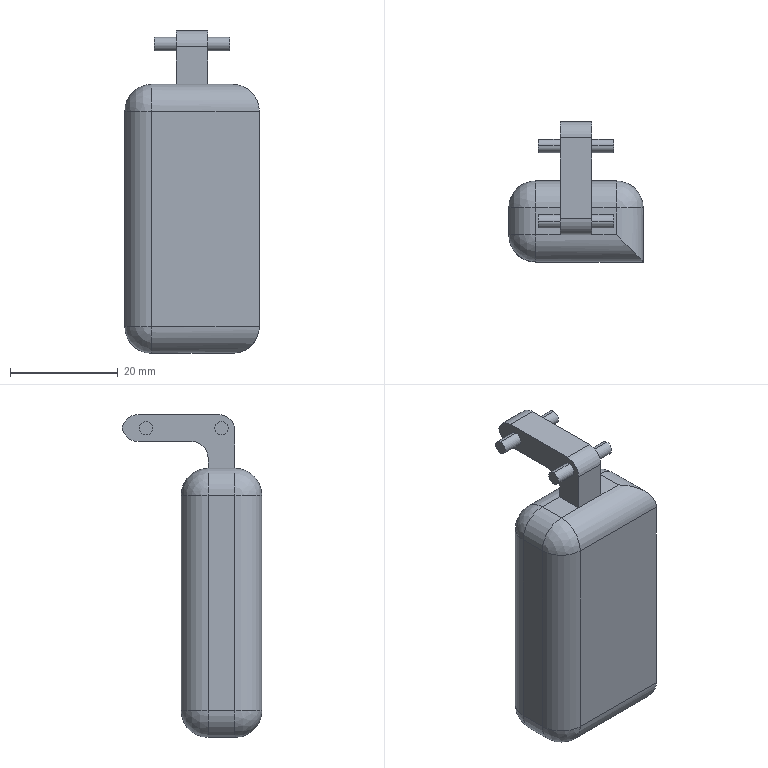Part | SolidWorks | features ICE 3, Fillet 2, Extrusion 1 | 1 solid | 46 faces | box 25 x 25.958 x 60 mm | volume 18052 mm3 | cylinder 23 | plane 17 | sphere 6 | commonest cylinder face diameters 10 x11 2.5 x8 6 x4
STEP:
#1=CARTESIAN_POINT('',(7.,14.,6.255));
#2=VERTEX_POINT('',#1);
#3=CARTESIAN_POINT('',(7.,14.,8.755));
#4=VERTEX_POINT('',#3);
#5=CARTESIAN_POINT('',(7.,14.,7.505));
#6=DIRECTION('',(1.,0.,0.));
#7=DIRECTION('',(0.,0.,-1.));
#8=AXIS2_PLACEMENT_3D('',#5,#6,#7);
#9=CIRCLE('',#8,1.25);
#10=EDGE_CURVE('',#2,#4,#9,.T.);
#11=ORIENTED_EDGE('',*,*,#10,.F.);
#12=CARTESIAN_POINT('',(2.916,14.,6.255));
#13=VERTEX_POINT('',#12);
#14=CARTESIAN_POINT('',(7.,14.,6.255));
#15=DIRECTION('',(-1.,0.,0.));
#16=VECTOR('',#15,1000.);
#17=LINE('',#14,#16);
#18=EDGE_CURVE('',#2,#13,#17,.T.);
#19=ORIENTED_EDGE('',*,*,#18,.T.);
#20=CARTESIAN_POINT('',(2.916,14.,8.755));
#21=VERTEX_POINT('',#20);
#22=CARTESIAN_POINT('',(2.916,14.,7.505));
#23=DIRECTION('',(1.,0.,0.));
#24=DIRECTION('',(0.,0.,1.));
#25=AXIS2_PLACEMENT_3D('',#22,#23,#24);
#26=CIRCLE('',#25,1.25);
#27=EDGE_CURVE('',#13,#21,#26,.T.);
#28=ORIENTED_EDGE('',*,*,#27,.T.);
#29=CARTESIAN_POINT('',(7.,14.,8.755));
#30=DIRECTION('',(-1.,0.,0.));
#31=VECTOR('',#30,1000.);
#32=LINE('',#29,#31);
#33=EDGE_CURVE('',#4,#21,#32,.T.);
#34=ORIENTED_EDGE('',*,*,#33,.F.);
#35=EDGE_LOOP('',(#11,#19,#28,#34));
#36=FACE_OUTER_BOUND('',#35,.T.);
#37=CARTESIAN_POINT('',(7.,14.,7.505));
#38=DIRECTION('',(-1.,0.,0.));
#39=DIRECTION('',(0.,0.,1.));
#40=AXIS2_PLACEMENT_3D('',#37,#38,#39);
#41=CYLINDRICAL_SURFACE('',#40,1.25);
#42=ADVANCED_FACE('',(#36),#41,.T.);
#43=CARTESIAN_POINT('',(-2.916,14.,8.755));
#44=VERTEX_POINT('',#43);
#45=CARTESIAN_POINT('',(-2.916,14.,6.255));
#46=VERTEX_POINT('',#45);
#47=CARTESIAN_POINT('',(-2.916,14.,7.505));
#48=DIRECTION('',(-1.,0.,0.));
#49=DIRECTION('',(0.,0.,-1.));
#50=AXIS2_PLACEMENT_3D('',#47,#48,#49);
#51=CIRCLE('',#50,1.25);
#52=EDGE_CURVE('',#44,#46,#51,.T.);
#53=ORIENTED_EDGE('',*,*,#52,.T.);
#54=CARTESIAN_POINT('',(-7.,14.,6.255));
#55=VERTEX_POINT('',#54);
#56=CARTESIAN_POINT('',(7.,14.,6.255));
#57=DIRECTION('',(-1.,0.,0.));
#58=VECTOR('',#57,1000.);
#59=LINE('',#56,#58);
#60=EDGE_CURVE('',#46,#55,#59,.T.);
#61=ORIENTED_EDGE('',*,*,#60,.T.);
#62=CARTESIAN_POINT('',(-7.,14.,8.755));
#63=VERTEX_POINT('',#62);
#64=CARTESIAN_POINT('',(-7.,14.,7.505));
#65=DIRECTION('',(1.,0.,0.));
#66=DIRECTION('',(0.,0.,-1.));
#67=AXIS2_PLACEMENT_3D('',#64,#65,#66);
#68=CIRCLE('',#67,1.25);
#69=EDGE_CURVE('',#55,#63,#68,.T.);
#70=ORIENTED_EDGE('',*,*,#69,.T.);
#71=CARTESIAN_POINT('',(7.,14.,8.755));
#72=DIRECTION('',(-1.,0.,0.));
#73=VECTOR('',#72,1000.);
#74=LINE('',#71,#73);
#75=EDGE_CURVE('',#44,#63,#74,.T.);
#76=ORIENTED_EDGE('',*,*,#75,.F.);
#77=EDGE_LOOP('',(#53,#61,#70,#76));
#78=FACE_OUTER_BOUND('',#77,.T.);
#79=CARTESIAN_POINT('',(7.,14.,7.505));
#80=DIRECTION('',(-1.,0.,0.));
#81=DIRECTION('',(0.,0.,1.));
#82=AXIS2_PLACEMENT_3D('',#79,#80,#81);
#83=CYLINDRICAL_SURFACE('',#82,1.25);
#84=ADVANCED_FACE('',(#78),#83,.T.);
#85=CARTESIAN_POINT('',(7.,0.,6.255));
#86=VERTEX_POINT('',#85);
#87=CARTESIAN_POINT('',(7.,0.,8.755));
#88=VERTEX_POINT('',#87);
#89=CARTESIAN_POINT('',(7.,0.,7.505));
#90=DIRECTION('',(1.,0.,0.));
#91=DIRECTION('',(0.,0.,-1.));
#92=AXIS2_PLACEMENT_3D('',#89,#90,#91);
#93=CIRCLE('',#92,1.25);
#94=EDGE_CURVE('',#86,#88,#93,.T.);
#95=ORIENTED_EDGE('',*,*,#94,.F.);
#96=CARTESIAN_POINT('',(2.916,0.,6.255));
#97=VERTEX_POINT('',#96);
#98=CARTESIAN_POINT('',(7.,0.,6.255));
#99=DIRECTION('',(-1.,0.,0.));
#100=VECTOR('',#99,1000.);
#101=LINE('',#98,#100);
#102=EDGE_CURVE('',#86,#97,#101,.T.);
#103=ORIENTED_EDGE('',*,*,#102,.T.);
#104=CARTESIAN_POINT('',(2.916,0.,8.755));
#105=VERTEX_POINT('',#104);
#106=CARTESIAN_POINT('',(2.916,0.,7.505));
#107=DIRECTION('',(1.,0.,0.));
#108=DIRECTION('',(0.,0.,1.));
#109=AXIS2_PLACEMENT_3D('',#106,#107,#108);
#110=CIRCLE('',#109,1.25);
#111=EDGE_CURVE('',#97,#105,#110,.T.);
#112=ORIENTED_EDGE('',*,*,#111,.T.);
#113=CARTESIAN_POINT('',(7.,0.,8.755));
#114=DIRECTION('',(-1.,0.,0.));
#115=VECTOR('',#114,1000.);
#116=LINE('',#113,#115);
#117=EDGE_CURVE('',#88,#105,#116,.T.);
#118=ORIENTED_EDGE('',*,*,#117,.F.);
#119=EDGE_LOOP('',(#95,#103,#112,#118));
#120=FACE_OUTER_BOUND('',#119,.T.);
#121=CARTESIAN_POINT('',(7.,0.,7.505));
#122=DIRECTION('',(-1.,0.,0.));
#123=DIRECTION('',(0.,0.,1.));
#124=AXIS2_PLACEMENT_3D('',#121,#122,#123);
#125=CYLINDRICAL_SURFACE('',#124,1.25);
#126=ADVANCED_FACE('',(#120),#125,.T.);
#127=CARTESIAN_POINT('',(-2.916,0.,8.755));
#128=VERTEX_POINT('',#127);
#129=CARTESIAN_POINT('',(-2.916,0.,6.255));
#130=VERTEX_POINT('',#129);
#131=CARTESIAN_POINT('',(-2.916,0.,7.505));
#132=DIRECTION('',(-1.,0.,0.));
#133=DIRECTION('',(0.,0.,-1.));
#134=AXIS2_PLACEMENT_3D('',#131,#132,#133);
#135=CIRCLE('',#134,1.25);
#136=EDGE_CURVE('',#128,#130,#135,.T.);
#137=ORIENTED_EDGE('',*,*,#136,.T.);
#138=CARTESIAN_POINT('',(-7.,0.,6.255));
#139=VERTEX_POINT('',#138);
#140=CARTESIAN_POINT('',(7.,0.,6.255));
#141=DIRECTION('',(-1.,0.,0.));
#142=VECTOR('',#141,1000.);
#143=LINE('',#140,#142);
#144=EDGE_CURVE('',#130,#139,#143,.T.);
#145=ORIENTED_EDGE('',*,*,#144,.T.);
#146=CARTESIAN_POINT('',(-7.,0.,8.755));
#147=VERTEX_POINT('',#146);
#148=CARTESIAN_POINT('',(-7.,0.,7.505));
#149=DIRECTION('',(1.,0.,0.));
#150=DIRECTION('',(0.,0.,-1.));
#151=AXIS2_PLACEMENT_3D('',#148,#149,#150);
#152=CIRCLE('',#151,1.25);
#153=EDGE_CURVE('',#139,#147,#152,.T.);
#154=ORIENTED_EDGE('',*,*,#153,.T.);
#155=CARTESIAN_POINT('',(7.,0.,8.755));
#156=DIRECTION('',(-1.,0.,0.));
#157=VECTOR('',#156,1000.);
#158=LINE('',#155,#157);
#159=EDGE_CURVE('',#128,#147,#158,.T.);
#160=ORIENTED_EDGE('',*,*,#159,.F.);
#161=EDGE_LOOP('',(#137,#145,#154,#160));
#162=FACE_OUTER_BOUND('',#161,.T.);
#163=CARTESIAN_POINT('',(7.,0.,7.505));
#164=DIRECTION('',(-1.,0.,0.));
#165=DIRECTION('',(0.,0.,1.));
#166=AXIS2_PLACEMENT_3D('',#163,#164,#165);
#167=CYLINDRICAL_SURFACE('',#166,1.25);
#168=ADVANCED_FACE('',(#162),#167,.T.);
#169=CARTESIAN_POINT('',(-2.916,2.5,2.));
#170=VERTEX_POINT('',#169);
#171=CARTESIAN_POINT('',(-2.916,2.5,0.));
#172=VERTEX_POINT('',#171);
#173=CARTESIAN_POINT('',(-2.916,2.5,10.));
#174=DIRECTION('',(0.,0.,-1.));
#175=VECTOR('',#174,1000.);
#176=LINE('',#173,#175);
#177=EDGE_CURVE('',#170,#172,#176,.T.);
#178=ORIENTED_EDGE('',*,*,#177,.F.);
#179=CARTESIAN_POINT('',(2.916,2.5,2.));
#180=VERTEX_POINT('',#179);
#181=CARTESIAN_POINT('',(2.916,2.5,2.));
#182=DIRECTION('',(1.,0.,0.));
#183=VECTOR('',#182,1000.);
#184=LINE('',#181,#183);
#185=EDGE_CURVE('',#170,#180,#184,.T.);
#186=ORIENTED_EDGE('',*,*,#185,.T.);
#187=CARTESIAN_POINT('',(2.916,2.5,0.));
#188=VERTEX_POINT('',#187);
#189=CARTESIAN_POINT('',(2.916,2.5,10.));
#190=DIRECTION('',(0.,0.,-1.));
#191=VECTOR('',#190,1000.);
#192=LINE('',#189,#191);
#193=EDGE_CURVE('',#180,#188,#192,.T.);
#194=ORIENTED_EDGE('',*,*,#193,.T.);
#195=CARTESIAN_POINT('',(-2.916,2.5,0.));
#196=DIRECTION('',(-1.,0.,0.));
#197=VECTOR('',#196,1000.);
#198=LINE('',#195,#197);
#199=EDGE_CURVE('',#188,#172,#198,.T.);
#200=ORIENTED_EDGE('',*,*,#199,.T.);
#201=EDGE_LOOP('',(#178,#186,#194,#200));
#202=FACE_OUTER_BOUND('',#201,.T.);
#203=CARTESIAN_POINT('',(-2.916,2.5,10.));
#204=DIRECTION('',(0.,-1.,0.));
#205=DIRECTION('',(0.,0.,-1.));
#206=AXIS2_PLACEMENT_3D('',#203,#204,#205);
#207=PLANE('',#206);
#208=ADVANCED_FACE('',(#202),#207,.F.);
#209=CARTESIAN_POINT('',(7.5,2.5,0.));
#210=VERTEX_POINT('',#209);
#211=CARTESIAN_POINT('',(0.,2.5,0.));
#212=DIRECTION('',(-1.,0.,0.));
#213=VECTOR('',#212,1000.);
#214=LINE('',#211,#213);
#215=EDGE_CURVE('',#210,#188,#214,.T.);
#216=ORIENTED_EDGE('',*,*,#215,.T.);
#217=CARTESIAN_POINT('',(2.916,-2.5,0.));
#218=VERTEX_POINT('',#217);
#219=CARTESIAN_POINT('',(2.916,2.5,0.));
#220=DIRECTION('',(0.,1.,0.));
#221=VECTOR('',#220,1000.);
#222=LINE('',#219,#221);
#223=EDGE_CURVE('',#218,#188,#222,.T.);
#224=ORIENTED_EDGE('',*,*,#223,.F.);
#225=CARTESIAN_POINT('',(7.5,-2.5,0.));
#226=VERTEX_POINT('',#225);
#227=CARTESIAN_POINT('',(0.,-2.5,0.));
#228=DIRECTION('',(1.,0.,0.));
#229=VECTOR('',#228,1000.);
#230=LINE('',#227,#229);
#231=EDGE_CURVE('',#218,#226,#230,.T.);
#232=ORIENTED_EDGE('',*,*,#231,.T.);
#233=CARTESIAN_POINT('',(7.5,0.,0.));
#234=DIRECTION('',(0.,1.,0.));
#235=VECTOR('',#234,1000.);
#236=LINE('',#233,#235);
#237=EDGE_CURVE('',#226,#210,#236,.T.);
#238=ORIENTED_EDGE('',*,*,#237,.T.);
#239=EDGE_LOOP('',(#216,#224,#232,#238));
#240=FACE_OUTER_BOUND('',#239,.T.);
#241=CARTESIAN_POINT('',(0.,0.,0.));
#242=DIRECTION('',(0.,0.,1.));
#243=DIRECTION('',(1.,0.,0.));
#244=AXIS2_PLACEMENT_3D('',#241,#242,#243);
#245=PLANE('',#244);
#246=ADVANCED_FACE('',(#240),#245,.T.);
#247=CARTESIAN_POINT('',(-7.5,-2.5,0.));
#248=VERTEX_POINT('',#247);
#249=CARTESIAN_POINT('',(-2.916,-2.5,0.));
#250=VERTEX_POINT('',#249);
#251=CARTESIAN_POINT('',(0.,-2.5,0.));
#252=DIRECTION('',(1.,0.,0.));
#253=VECTOR('',#252,1000.);
#254=LINE('',#251,#253);
#255=EDGE_CURVE('',#248,#250,#254,.T.);
#256=ORIENTED_EDGE('',*,*,#255,.T.);
#257=CARTESIAN_POINT('',(-2.916,2.5,0.));
#258=DIRECTION('',(0.,-1.,0.));
#259=VECTOR('',#258,1000.);
#260=LINE('',#257,#259);
#261=EDGE_CURVE('',#172,#250,#260,.T.);
#262=ORIENTED_EDGE('',*,*,#261,.F.);
#263=CARTESIAN_POINT('',(-7.5,2.5,0.));
#264=VERTEX_POINT('',#263);
#265=CARTESIAN_POINT('',(0.,2.5,0.));
#266=DIRECTION('',(-1.,0.,0.));
#267=VECTOR('',#266,1000.);
#268=LINE('',#265,#267);
#269=EDGE_CURVE('',#172,#264,#268,.T.);
#270=ORIENTED_EDGE('',*,*,#269,.T.);
#271=CARTESIAN_POINT('',(-7.5,0.,0.));
#272=DIRECTION('',(0.,-1.,0.));
#273=VECTOR('',#272,1000.);
#274=LINE('',#271,#273);
#275=EDGE_CURVE('',#264,#248,#274,.T.);
#276=ORIENTED_EDGE('',*,*,#275,.T.);
#277=EDGE_LOOP('',(#256,#262,#270,#276));
#278=FACE_OUTER_BOUND('',#277,.T.);
#279=CARTESIAN_POINT('',(0.,0.,0.));
#280=DIRECTION('',(0.,0.,1.));
#281=DIRECTION('',(1.,0.,0.));
#282=AXIS2_PLACEMENT_3D('',#279,#280,#281);
#283=PLANE('',#282);
#284=ADVANCED_FACE('',(#278),#283,.T.);
#285=CARTESIAN_POINT('',(12.5,2.5,-45.));
#286=VERTEX_POINT('',#285);
#287=CARTESIAN_POINT('',(12.5,2.5,-5.));
#288=VERTEX_POINT('',#287);
#289=CARTESIAN_POINT('',(12.5,2.5,-50.));
#290=DIRECTION('',(0.,0.,1.));
#291=VECTOR('',#290,1000.);
#292=LINE('',#289,#291);
#293=EDGE_CURVE('',#286,#288,#292,.T.);
#294=ORIENTED_EDGE('',*,*,#293,.T.);
#295=CARTESIAN_POINT('',(12.5,-7.5,-5.));
#296=VERTEX_POINT('',#295);
#297=CARTESIAN_POINT('',(12.5,7.5,-5.));
#298=DIRECTION('',(0.,-1.,0.));
#299=VECTOR('',#298,1000.);
#300=LINE('',#297,#299);
#301=EDGE_CURVE('',#288,#296,#300,.T.);
#302=ORIENTED_EDGE('',*,*,#301,.T.);
#303=CARTESIAN_POINT('',(12.5,-7.5,-45.));
#304=VERTEX_POINT('',#303);
#305=CARTESIAN_POINT('',(12.5,-7.5,-50.));
#306=DIRECTION('',(0.,0.,1.));
#307=VECTOR('',#306,1000.);
#308=LINE('',#305,#307);
#309=EDGE_CURVE('',#304,#296,#308,.T.);
#310=ORIENTED_EDGE('',*,*,#309,.F.);
#311=CARTESIAN_POINT('',(12.5,7.5,-45.));
#312=DIRECTION('',(0.,1.,0.));
#313=VECTOR('',#312,1000.);
#314=LINE('',#311,#313);
#315=EDGE_CURVE('',#304,#286,#314,.T.);
#316=ORIENTED_EDGE('',*,*,#315,.T.);
#317=EDGE_LOOP('',(#294,#302,#310,#316));
#318=FACE_OUTER_BOUND('',#317,.T.);
#319=CARTESIAN_POINT('',(12.5,7.5,-50.));
#320=DIRECTION('',(1.,0.,0.));
#321=DIRECTION('',(0.,1.,0.));
#322=AXIS2_PLACEMENT_3D('',#319,#320,#321);
#323=PLANE('',#322);
#324=ADVANCED_FACE('',(#318),#323,.T.);
#325=ORIENTED_EDGE('',*,*,#309,.T.);
#326=CARTESIAN_POINT('',(-7.5,-7.5,-5.));
#327=VERTEX_POINT('',#326);
#328=CARTESIAN_POINT('',(-12.5,-7.5,-5.));
#329=DIRECTION('',(-1.,0.,0.));
#330=VECTOR('',#329,1000.);
#331=LINE('',#328,#330);
#332=EDGE_CURVE('',#296,#327,#331,.T.);
#333=ORIENTED_EDGE('',*,*,#332,.T.);
#334=CARTESIAN_POINT('',(-7.5,-7.5,-45.));
#335=VERTEX_POINT('',#334);
#336=CARTESIAN_POINT('',(-7.5,-7.5,-50.));
#337=DIRECTION('',(0.,0.,-1.));
#338=VECTOR('',#337,1000.);
#339=LINE('',#336,#338);
#340=EDGE_CURVE('',#327,#335,#339,.T.);
#341=ORIENTED_EDGE('',*,*,#340,.T.);
#342=CARTESIAN_POINT('',(12.5,-7.5,-45.));
#343=DIRECTION('',(1.,0.,0.));
#344=VECTOR('',#343,1000.);
#345=LINE('',#342,#344);
#346=EDGE_CURVE('',#335,#304,#345,.T.);
#347=ORIENTED_EDGE('',*,*,#346,.T.);
#348=EDGE_LOOP('',(#325,#333,#341,#347));
#349=FACE_OUTER_BOUND('',#348,.T.);
#350=CARTESIAN_POINT('',(-12.5,-7.5,-50.));
#351=DIRECTION('',(0.,-1.,0.));
#352=DIRECTION('',(0.,0.,-1.));
#353=AXIS2_PLACEMENT_3D('',#350,#351,#352);
#354=PLANE('',#353);
#355=ADVANCED_FACE('',(#349),#354,.T.);
#356=CARTESIAN_POINT('',(-12.5,-2.5,-45.));
#357=VERTEX_POINT('',#356);
#358=CARTESIAN_POINT('',(-12.5,-2.5,-5.));
#359=VERTEX_POINT('',#358);
#360=CARTESIAN_POINT('',(-12.5,-2.5,-50.));
#361=DIRECTION('',(0.,0.,1.));
#362=VECTOR('',#361,1000.);
#363=LINE('',#360,#362);
#364=EDGE_CURVE('',#357,#359,#363,.T.);
#365=ORIENTED_EDGE('',*,*,#364,.T.);
#366=CARTESIAN_POINT('',(-12.5,2.5,-5.));
#367=VERTEX_POINT('',#366);
#368=CARTESIAN_POINT('',(-12.5,7.5,-5.));
#369=DIRECTION('',(0.,1.,0.));
#370=VECTOR('',#369,1000.);
#371=LINE('',#368,#370);
#372=EDGE_CURVE('',#359,#367,#371,.T.);
#373=ORIENTED_EDGE('',*,*,#372,.T.);
#374=CARTESIAN_POINT('',(-12.5,2.5,-45.));
#375=VERTEX_POINT('',#374);
#376=CARTESIAN_POINT('',(-12.5,2.5,-50.));
#377=DIRECTION('',(0.,0.,-1.));
#378=VECTOR('',#377,1000.);
#379=LINE('',#376,#378);
#380=EDGE_CURVE('',#367,#375,#379,.T.);
#381=ORIENTED_EDGE('',*,*,#380,.T.);
#382=CARTESIAN_POINT('',(-12.5,-7.5,-45.));
#383=DIRECTION('',(0.,-1.,0.));
#384=VECTOR('',#383,1000.);
#385=LINE('',#382,#384);
#386=EDGE_CURVE('',#375,#357,#385,.T.);
#387=ORIENTED_EDGE('',*,*,#386,.T.);
#388=EDGE_LOOP('',(#365,#373,#381,#387));
#389=FACE_OUTER_BOUND('',#388,.T.);
#390=CARTESIAN_POINT('',(-12.5,7.5,-50.));
#391=DIRECTION('',(-1.,0.,0.));
#392=DIRECTION('',(0.,-1.,0.));
#393=AXIS2_PLACEMENT_3D('',#390,#391,#392);
#394=PLANE('',#393);
#395=ADVANCED_FACE('',(#389),#394,.T.);
#396=CARTESIAN_POINT('',(7.5,7.5,-45.));
#397=VERTEX_POINT('',#396);
#398=CARTESIAN_POINT('',(-7.5,7.5,-45.));
#399=VERTEX_POINT('',#398);
#400=CARTESIAN_POINT('',(-12.5,7.5,-45.));
#401=DIRECTION('',(-1.,0.,0.));
#402=VECTOR('',#401,1000.);
#403=LINE('',#400,#402);
#404=EDGE_CURVE('',#397,#399,#403,.T.);
#405=ORIENTED_EDGE('',*,*,#404,.T.);
#406=CARTESIAN_POINT('',(-7.5,7.5,-5.));
#407=VERTEX_POINT('',#406);
#408=CARTESIAN_POINT('',(-7.5,7.5,-50.));
#409=DIRECTION('',(0.,0.,1.));
#410=VECTOR('',#409,1000.);
#411=LINE('',#408,#410);
#412=EDGE_CURVE('',#399,#407,#411,.T.);
#413=ORIENTED_EDGE('',*,*,#412,.T.);
#414=CARTESIAN_POINT('',(7.5,7.5,-5.));
#415=VERTEX_POINT('',#414);
#416=CARTESIAN_POINT('',(-12.5,7.5,-5.));
#417=DIRECTION('',(1.,0.,0.));
#418=VECTOR('',#417,1000.);
#419=LINE('',#416,#418);
#420=EDGE_CURVE('',#407,#415,#419,.T.);
#421=ORIENTED_EDGE('',*,*,#420,.T.);
#422=CARTESIAN_POINT('',(7.5,7.5,-50.));
#423=DIRECTION('',(0.,0.,-1.));
#424=VECTOR('',#423,1000.);
#425=LINE('',#422,#424);
#426=EDGE_CURVE('',#415,#397,#425,.T.);
#427=ORIENTED_EDGE('',*,*,#426,.T.);
#428=EDGE_LOOP('',(#405,#413,#421,#427));
#429=FACE_OUTER_BOUND('',#428,.T.);
#430=CARTESIAN_POINT('',(-12.5,7.5,-50.));
#431=DIRECTION('',(0.,1.,0.));
#432=DIRECTION('',(0.,0.,1.));
#433=AXIS2_PLACEMENT_3D('',#430,#431,#432);
#434=PLANE('',#433);
#435=ADVANCED_FACE('',(#429),#434,.T.);
#436=CARTESIAN_POINT('',(7.5,2.5,-50.));
#437=VERTEX_POINT('',#436);
#438=CARTESIAN_POINT('',(7.5,-2.5,-50.));
#439=VERTEX_POINT('',#438);
#440=CARTESIAN_POINT('',(7.5,-7.5,-50.));
#441=DIRECTION('',(0.,-1.,0.));
#442=VECTOR('',#441,1000.);
#443=LINE('',#440,#442);
#444=EDGE_CURVE('',#437,#439,#443,.T.);
#445=ORIENTED_EDGE('',*,*,#444,.T.);
#446=CARTESIAN_POINT('',(-7.5,-2.5,-50.));
#447=VERTEX_POINT('',#446);
#448=CARTESIAN_POINT('',(-12.5,-2.5,-50.));
#449=DIRECTION('',(-1.,0.,0.));
#450=VECTOR('',#449,1000.);
#451=LINE('',#448,#450);
#452=EDGE_CURVE('',#439,#447,#451,.T.);
#453=ORIENTED_EDGE('',*,*,#452,.T.);
#454=CARTESIAN_POINT('',(-7.5,2.5,-50.));
#455=VERTEX_POINT('',#454);
#456=CARTESIAN_POINT('',(-7.5,7.5,-50.));
#457=DIRECTION('',(0.,1.,0.));
#458=VECTOR('',#457,1000.);
#459=LINE('',#456,#458);
#460=EDGE_CURVE('',#447,#455,#459,.T.);
#461=ORIENTED_EDGE('',*,*,#460,.T.);
#462=CARTESIAN_POINT('',(12.5,2.5,-50.));
#463=DIRECTION('',(1.,0.,0.));
#464=VECTOR('',#463,1000.);
#465=LINE('',#462,#464);
#466=EDGE_CURVE('',#455,#437,#465,.T.);
#467=ORIENTED_EDGE('',*,*,#466,.T.);
#468=EDGE_LOOP('',(#445,#453,#461,#467));
#469=FACE_OUTER_BOUND('',#468,.T.);
#470=CARTESIAN_POINT('',(0.,0.,-50.));
#471=DIRECTION('',(0.,0.,1.));
#472=DIRECTION('',(1.,0.,0.));
#473=AXIS2_PLACEMENT_3D('',#470,#471,#472);
#474=PLANE('',#473);
#475=ADVANCED_FACE('',(#469),#474,.F.);
#476=CARTESIAN_POINT('',(7.5,2.5,-45.));
#477=DIRECTION('',(0.,0.,1.));
#478=DIRECTION('',(-1.,0.,0.));
#479=AXIS2_PLACEMENT_3D('',#476,#477,#478);
#480=CIRCLE('',#479,5.);
#481=EDGE_CURVE('',#286,#397,#480,.T.);
#482=ORIENTED_EDGE('',*,*,#481,.F.);
#483=CARTESIAN_POINT('',(7.5,2.5,-45.));
#484=DIRECTION('',(0.,-1.,0.));
#485=DIRECTION('',(-1.,0.,0.));
#486=AXIS2_PLACEMENT_3D('',#483,#484,#485);
#487=CIRCLE('',#486,5.);
#488=EDGE_CURVE('',#437,#286,#487,.T.);
#489=ORIENTED_EDGE('',*,*,#488,.F.);
#490=CARTESIAN_POINT('',(7.5,2.5,-45.));
#491=DIRECTION('',(-1.,0.,0.));
#492=DIRECTION('',(0.,0.,-1.));
#493=AXIS2_PLACEMENT_3D('',#490,#491,#492);
#494=CIRCLE('',#493,5.);
#495=EDGE_CURVE('',#397,#437,#494,.T.);
#496=ORIENTED_EDGE('',*,*,#495,.F.);
#497=EDGE_LOOP('',(#482,#489,#496));
#498=FACE_OUTER_BOUND('',#497,.T.);
#499=CARTESIAN_POINT('',(7.5,2.5,-45.));
#500=DIRECTION('',(0.,1.,0.));
#501=DIRECTION('',(-1.,0.,0.));
#502=AXIS2_PLACEMENT_3D('',#499,#500,#501);
#503=SPHERICAL_SURFACE('',#502,5.);
#504=ADVANCED_FACE('',(#498),#503,.T.);
#505=ORIENTED_EDGE('',*,*,#488,.T.);
#506=ORIENTED_EDGE('',*,*,#315,.F.);
#507=CARTESIAN_POINT('',(7.5,-2.5,-50.));
#508=CARTESIAN_POINT('',(10.429,-5.429,-50.));
#509=CARTESIAN_POINT('',(12.5,-7.5,-47.929));
#510=CARTESIAN_POINT('',(12.5,-7.5,-45.));
#511=(BOUNDED_CURVE()B_SPLINE_CURVE(3,(#507,#508,#509,#510),.UNSPECIFIED.,.F.,.T.)B_SPLINE_CURVE_WITH_KNOTS((4,4),(4.712,6.283),.UNSPECIFIED.)CURVE()GEOMETRIC_REPRESENTATION_ITEM()RATIONAL_B_SPLINE_CURVE((1.,0.8047,0.8047,1.))REPRESENTATION_ITEM(''));
#512=EDGE_CURVE('',#439,#304,#511,.T.);
#513=ORIENTED_EDGE('',*,*,#512,.F.);
#514=ORIENTED_EDGE('',*,*,#444,.F.);
#515=EDGE_LOOP('',(#505,#506,#513,#514));
#516=FACE_OUTER_BOUND('',#515,.T.);
#517=CARTESIAN_POINT('',(7.5,7.5,-45.));
#518=DIRECTION('',(0.,-1.,0.));
#519=DIRECTION('',(1.,0.,0.));
#520=AXIS2_PLACEMENT_3D('',#517,#518,#519);
#521=CYLINDRICAL_SURFACE('',#520,5.);
#522=ADVANCED_FACE('',(#516),#521,.T.);
#523=ORIENTED_EDGE('',*,*,#495,.T.);
#524=ORIENTED_EDGE('',*,*,#466,.F.);
#525=CARTESIAN_POINT('',(-7.5,2.5,-45.));
#526=DIRECTION('',(-1.,0.,0.));
#527=DIRECTION('',(0.,0.,1.));
#528=AXIS2_PLACEMENT_3D('',#525,#526,#527);
#529=CIRCLE('',#528,5.);
#530=EDGE_CURVE('',#399,#455,#529,.T.);
#531=ORIENTED_EDGE('',*,*,#530,.F.);
#532=ORIENTED_EDGE('',*,*,#404,.F.);
#533=EDGE_LOOP('',(#523,#524,#531,#532));
#534=FACE_OUTER_BOUND('',#533,.T.);
#535=CARTESIAN_POINT('',(-12.5,2.5,-45.));
#536=DIRECTION('',(1.,0.,0.));
#537=DIRECTION('',(0.,0.,-1.));
#538=AXIS2_PLACEMENT_3D('',#535,#536,#537);
#539=CYLINDRICAL_SURFACE('',#538,5.);
#540=ADVANCED_FACE('',(#534),#539,.T.);
#541=ORIENTED_EDGE('',*,*,#481,.T.);
#542=ORIENTED_EDGE('',*,*,#426,.F.);
#543=CARTESIAN_POINT('',(7.5,2.5,-5.));
#544=DIRECTION('',(0.,0.,1.));
#545=DIRECTION('',(1.,0.,0.));
#546=AXIS2_PLACEMENT_3D('',#543,#544,#545);
#547=CIRCLE('',#546,5.);
#548=EDGE_CURVE('',#288,#415,#547,.T.);
#549=ORIENTED_EDGE('',*,*,#548,.F.);
#550=ORIENTED_EDGE('',*,*,#293,.F.);
#551=EDGE_LOOP('',(#541,#542,#549,#550));
#552=FACE_OUTER_BOUND('',#551,.T.);
#553=CARTESIAN_POINT('',(7.5,2.5,-50.));
#554=DIRECTION('',(0.,0.,1.));
#555=DIRECTION('',(1.,0.,0.));
#556=AXIS2_PLACEMENT_3D('',#553,#554,#555);
#557=CYLINDRICAL_SURFACE('',#556,5.);
#558=ADVANCED_FACE('',(#552),#557,.T.);
#559=ORIENTED_EDGE('',*,*,#512,.T.);
#560=ORIENTED_EDGE('',*,*,#346,.F.);
#561=CARTESIAN_POINT('',(-7.5,-2.5,-45.));
#562=DIRECTION('',(-1.,0.,0.));
#563=DIRECTION('',(0.,0.,1.));
#564=AXIS2_PLACEMENT_3D('',#561,#562,#563);
#565=CIRCLE('',#564,5.);
#566=EDGE_CURVE('',#447,#335,#565,.T.);
#567=ORIENTED_EDGE('',*,*,#566,.F.);
#568=ORIENTED_EDGE('',*,*,#452,.F.);
#569=EDGE_LOOP('',(#559,#560,#567,#568));
#570=FACE_OUTER_BOUND('',#569,.T.);
#571=CARTESIAN_POINT('',(-12.5,-2.5,-45.));
#572=DIRECTION('',(-1.,0.,0.));
#573=DIRECTION('',(0.,0.,1.));
#574=AXIS2_PLACEMENT_3D('',#571,#572,#573);
#575=CYLINDRICAL_SURFACE('',#574,5.);
#576=ADVANCED_FACE('',(#570),#575,.T.);
#577=CARTESIAN_POINT('',(-7.5,2.5,-45.));
#578=DIRECTION('',(0.,1.,0.));
#579=DIRECTION('',(-1.,0.,0.));
#580=AXIS2_PLACEMENT_3D('',#577,#578,#579);
#581=CIRCLE('',#580,5.);
#582=EDGE_CURVE('',#455,#375,#581,.T.);
#583=ORIENTED_EDGE('',*,*,#582,.F.);
#584=ORIENTED_EDGE('',*,*,#460,.F.);
#585=CARTESIAN_POINT('',(-7.5,-2.5,-45.));
#586=DIRECTION('',(0.,-1.,0.));
#587=DIRECTION('',(1.,0.,0.));
#588=AXIS2_PLACEMENT_3D('',#585,#586,#587);
#589=CIRCLE('',#588,5.);
#590=EDGE_CURVE('',#357,#447,#589,.T.);
#591=ORIENTED_EDGE('',*,*,#590,.F.);
#592=ORIENTED_EDGE('',*,*,#386,.F.);
#593=EDGE_LOOP('',(#583,#584,#591,#592));
#594=FACE_OUTER_BOUND('',#593,.T.);
#595=CARTESIAN_POINT('',(-7.5,7.5,-45.));
#596=DIRECTION('',(0.,1.,0.));
#597=DIRECTION('',(-1.,0.,0.));
#598=AXIS2_PLACEMENT_3D('',#595,#596,#597);
#599=CYLINDRICAL_SURFACE('',#598,5.);
#600=ADVANCED_FACE('',(#594),#599,.T.);
#601=ORIENTED_EDGE('',*,*,#530,.T.);
#602=ORIENTED_EDGE('',*,*,#582,.T.);
#603=CARTESIAN_POINT('',(-7.5,2.5,-45.));
#604=DIRECTION('',(0.,0.,1.));
#605=DIRECTION('',(-1.,0.,0.));
#606=AXIS2_PLACEMENT_3D('',#603,#604,#605);
#607=CIRCLE('',#606,5.);
#608=EDGE_CURVE('',#399,#375,#607,.T.);
#609=ORIENTED_EDGE('',*,*,#608,.F.);
#610=EDGE_LOOP('',(#601,#602,#609));
#611=FACE_OUTER_BOUND('',#610,.T.);
#612=CARTESIAN_POINT('',(-7.5,2.5,-45.));
#613=DIRECTION('',(0.,1.,0.));
#614=DIRECTION('',(-1.,0.,0.));
#615=AXIS2_PLACEMENT_3D('',#612,#613,#614);
#616=SPHERICAL_SURFACE('',#615,5.);
#617=ADVANCED_FACE('',(#611),#616,.T.);
#618=CARTESIAN_POINT('',(7.5,2.5,-5.));
#619=DIRECTION('',(-1.,0.,0.));
#620=DIRECTION('',(0.,0.,-1.));
#621=AXIS2_PLACEMENT_3D('',#618,#619,#620);
#622=CIRCLE('',#621,5.);
#623=EDGE_CURVE('',#210,#415,#622,.T.);
#624=ORIENTED_EDGE('',*,*,#623,.F.);
#625=CARTESIAN_POINT('',(7.5,2.5,-5.));
#626=DIRECTION('',(0.,-1.,0.));
#627=DIRECTION('',(-1.,0.,0.));
#628=AXIS2_PLACEMENT_3D('',#625,#626,#627);
#629=CIRCLE('',#628,5.);
#630=EDGE_CURVE('',#288,#210,#629,.T.);
#631=ORIENTED_EDGE('',*,*,#630,.F.);
#632=ORIENTED_EDGE('',*,*,#548,.T.);
#633=EDGE_LOOP('',(#624,#631,#632));
#634=FACE_OUTER_BOUND('',#633,.T.);
#635=CARTESIAN_POINT('',(7.5,2.5,-5.));
#636=DIRECTION('',(0.,0.,1.));
#637=DIRECTION('',(0.,1.,0.));
#638=AXIS2_PLACEMENT_3D('',#635,#636,#637);
#639=SPHERICAL_SURFACE('',#638,5.);
#640=ADVANCED_FACE('',(#634),#639,.T.);
#641=ORIENTED_EDGE('',*,*,#630,.T.);
#642=ORIENTED_EDGE('',*,*,#237,.F.);
#643=CARTESIAN_POINT('',(12.5,-7.5,-5.));
#644=CARTESIAN_POINT('',(12.5,-7.5,-2.071));
#645=CARTESIAN_POINT('',(10.429,-5.429,0.));
#646=CARTESIAN_POINT('',(7.5,-2.5,0.));
#647=(BOUNDED_CURVE()B_SPLINE_CURVE(3,(#643,#644,#645,#646),.UNSPECIFIED.,.F.,.F.)B_SPLINE_CURVE_WITH_KNOTS((4,4),(3.142,4.712),.UNSPECIFIED.)CURVE()GEOMETRIC_REPRESENTATION_ITEM()RATIONAL_B_SPLINE_CURVE((1.,0.8047,0.8047,1.))REPRESENTATION_ITEM(''));
#648=EDGE_CURVE('',#296,#226,#647,.T.);
#649=ORIENTED_EDGE('',*,*,#648,.F.);
#650=ORIENTED_EDGE('',*,*,#301,.F.);
#651=EDGE_LOOP('',(#641,#642,#649,#650));
#652=FACE_OUTER_BOUND('',#651,.T.);
#653=CARTESIAN_POINT('',(7.5,0.,-5.));
#654=DIRECTION('',(0.,1.,0.));
#655=DIRECTION('',(-1.,0.,0.));
#656=AXIS2_PLACEMENT_3D('',#653,#654,#655);
#657=CYLINDRICAL_SURFACE('',#656,5.);
#658=ADVANCED_FACE('',(#652),#657,.T.);
#659=ORIENTED_EDGE('',*,*,#590,.T.);
#660=ORIENTED_EDGE('',*,*,#566,.T.);
#661=CARTESIAN_POINT('',(-7.5,-2.5,-45.));
#662=DIRECTION('',(0.,0.,1.));
#663=DIRECTION('',(-1.,0.,0.));
#664=AXIS2_PLACEMENT_3D('',#661,#662,#663);
#665=CIRCLE('',#664,5.);
#666=EDGE_CURVE('',#357,#335,#665,.T.);
#667=ORIENTED_EDGE('',*,*,#666,.F.);
#668=EDGE_LOOP('',(#659,#660,#667));
#669=FACE_OUTER_BOUND('',#668,.T.);
#670=CARTESIAN_POINT('',(-7.5,-2.5,-45.));
#671=DIRECTION('',(0.,1.,0.));
#672=DIRECTION('',(-1.,0.,0.));
#673=AXIS2_PLACEMENT_3D('',#670,#671,#672);
#674=SPHERICAL_SURFACE('',#673,5.);
#675=ADVANCED_FACE('',(#669),#674,.T.);
#676=ORIENTED_EDGE('',*,*,#608,.T.);
#677=ORIENTED_EDGE('',*,*,#380,.F.);
#678=CARTESIAN_POINT('',(-7.5,2.5,-5.));
#679=DIRECTION('',(0.,0.,1.));
#680=DIRECTION('',(1.,0.,0.));
#681=AXIS2_PLACEMENT_3D('',#678,#679,#680);
#682=CIRCLE('',#681,5.);
#683=EDGE_CURVE('',#407,#367,#682,.T.);
#684=ORIENTED_EDGE('',*,*,#683,.F.);
#685=ORIENTED_EDGE('',*,*,#412,.F.);
#686=EDGE_LOOP('',(#676,#677,#684,#685));
#687=FACE_OUTER_BOUND('',#686,.T.);
#688=CARTESIAN_POINT('',(-7.5,2.5,-50.));
#689=DIRECTION('',(0.,0.,1.));
#690=DIRECTION('',(1.,0.,0.));
#691=AXIS2_PLACEMENT_3D('',#688,#689,#690);
#692=CYLINDRICAL_SURFACE('',#691,5.);
#693=ADVANCED_FACE('',(#687),#692,.T.);
#694=ORIENTED_EDGE('',*,*,#623,.T.);
#695=ORIENTED_EDGE('',*,*,#420,.F.);
#696=CARTESIAN_POINT('',(-7.5,2.5,-5.));
#697=DIRECTION('',(-1.,0.,0.));
#698=DIRECTION('',(0.,0.,1.));
#699=AXIS2_PLACEMENT_3D('',#696,#697,#698);
#700=CIRCLE('',#699,5.);
#701=EDGE_CURVE('',#264,#407,#700,.T.);
#702=ORIENTED_EDGE('',*,*,#701,.F.);
#703=ORIENTED_EDGE('',*,*,#269,.F.);
#704=ORIENTED_EDGE('',*,*,#199,.F.);
#705=ORIENTED_EDGE('',*,*,#215,.F.);
#706=EDGE_LOOP('',(#694,#695,#702,#703,#704,#705));
#707=FACE_OUTER_BOUND('',#706,.T.);
#708=CARTESIAN_POINT('',(0.,2.5,-5.));
#709=DIRECTION('',(-1.,0.,0.));
#710=DIRECTION('',(0.,0.,1.));
#711=AXIS2_PLACEMENT_3D('',#708,#709,#710);
#712=CYLINDRICAL_SURFACE('',#711,5.);
#713=ADVANCED_FACE('',(#707),#712,.T.);
#714=ORIENTED_EDGE('',*,*,#648,.T.);
#715=ORIENTED_EDGE('',*,*,#231,.F.);
#716=CARTESIAN_POINT('',(-2.916,-2.5,0.));
#717=DIRECTION('',(1.,0.,0.));
#718=VECTOR('',#717,1000.);
#719=LINE('',#716,#718);
#720=EDGE_CURVE('',#250,#218,#719,.T.);
#721=ORIENTED_EDGE('',*,*,#720,.F.);
#722=ORIENTED_EDGE('',*,*,#255,.F.);
#723=CARTESIAN_POINT('',(-7.5,-2.5,-5.));
#724=DIRECTION('',(-1.,0.,0.));
#725=DIRECTION('',(0.,0.,1.));
#726=AXIS2_PLACEMENT_3D('',#723,#724,#725);
#727=CIRCLE('',#726,5.);
#728=EDGE_CURVE('',#327,#248,#727,.T.);
#729=ORIENTED_EDGE('',*,*,#728,.F.);
#730=ORIENTED_EDGE('',*,*,#332,.F.);
#731=EDGE_LOOP('',(#714,#715,#721,#722,#729,#730));
#732=FACE_OUTER_BOUND('',#731,.T.);
#733=CARTESIAN_POINT('',(0.,-2.5,-5.));
#734=DIRECTION('',(1.,0.,0.));
#735=DIRECTION('',(0.,0.,-1.));
#736=AXIS2_PLACEMENT_3D('',#733,#734,#735);
#737=CYLINDRICAL_SURFACE('',#736,5.);
#738=ADVANCED_FACE('',(#732),#737,.T.);
#739=ORIENTED_EDGE('',*,*,#666,.T.);
#740=ORIENTED_EDGE('',*,*,#340,.F.);
#741=CARTESIAN_POINT('',(-7.5,-2.5,-5.));
#742=DIRECTION('',(0.,0.,1.));
#743=DIRECTION('',(1.,0.,0.));
#744=AXIS2_PLACEMENT_3D('',#741,#742,#743);
#745=CIRCLE('',#744,5.);
#746=EDGE_CURVE('',#359,#327,#745,.T.);
#747=ORIENTED_EDGE('',*,*,#746,.F.);
#748=ORIENTED_EDGE('',*,*,#364,.F.);
#749=EDGE_LOOP('',(#739,#740,#747,#748));
#750=FACE_OUTER_BOUND('',#749,.T.);
#751=CARTESIAN_POINT('',(-7.5,-2.5,-50.));
#752=DIRECTION('',(0.,0.,1.));
#753=DIRECTION('',(1.,0.,0.));
#754=AXIS2_PLACEMENT_3D('',#751,#752,#753);
#755=CYLINDRICAL_SURFACE('',#754,5.);
#756=ADVANCED_FACE('',(#750),#755,.T.);
#757=ORIENTED_EDGE('',*,*,#701,.T.);
#758=ORIENTED_EDGE('',*,*,#683,.T.);
#759=CARTESIAN_POINT('',(-7.5,2.5,-5.));
#760=DIRECTION('',(0.,-1.,0.));
#761=DIRECTION('',(-1.,0.,0.));
#762=AXIS2_PLACEMENT_3D('',#759,#760,#761);
#763=CIRCLE('',#762,5.);
#764=EDGE_CURVE('',#264,#367,#763,.T.);
#765=ORIENTED_EDGE('',*,*,#764,.F.);
#766=EDGE_LOOP('',(#757,#758,#765));
#767=FACE_OUTER_BOUND('',#766,.T.);
#768=CARTESIAN_POINT('',(-7.5,2.5,-5.));
#769=DIRECTION('',(1.,0.,0.));
#770=DIRECTION('',(0.,0.,1.));
#771=AXIS2_PLACEMENT_3D('',#768,#769,#770);
#772=SPHERICAL_SURFACE('',#771,5.);
#773=ADVANCED_FACE('',(#767),#772,.T.);
#774=ORIENTED_EDGE('',*,*,#746,.T.);
#775=ORIENTED_EDGE('',*,*,#728,.T.);
#776=CARTESIAN_POINT('',(-7.5,-2.5,-5.));
#777=DIRECTION('',(0.,1.,0.));
#778=DIRECTION('',(1.,0.,0.));
#779=AXIS2_PLACEMENT_3D('',#776,#777,#778);
#780=CIRCLE('',#779,5.);
#781=EDGE_CURVE('',#359,#248,#780,.T.);
#782=ORIENTED_EDGE('',*,*,#781,.F.);
#783=EDGE_LOOP('',(#774,#775,#782));
#784=FACE_OUTER_BOUND('',#783,.T.);
#785=CARTESIAN_POINT('',(-7.5,-2.5,-5.));
#786=DIRECTION('',(1.,0.,0.));
#787=DIRECTION('',(0.,0.,-1.));
#788=AXIS2_PLACEMENT_3D('',#785,#786,#787);
#789=SPHERICAL_SURFACE('',#788,5.);
#790=ADVANCED_FACE('',(#784),#789,.T.);
#791=ORIENTED_EDGE('',*,*,#764,.T.);
#792=ORIENTED_EDGE('',*,*,#372,.F.);
#793=ORIENTED_EDGE('',*,*,#781,.T.);
#794=ORIENTED_EDGE('',*,*,#275,.F.);
#795=EDGE_LOOP('',(#791,#792,#793,#794));
#796=FACE_OUTER_BOUND('',#795,.T.);
#797=CARTESIAN_POINT('',(-7.5,0.,-5.));
#798=DIRECTION('',(0.,-1.,0.));
#799=DIRECTION('',(1.,0.,0.));
#800=AXIS2_PLACEMENT_3D('',#797,#798,#799);
#801=CYLINDRICAL_SURFACE('',#800,5.);
#802=ADVANCED_FACE('',(#796),#801,.T.);
#803=CARTESIAN_POINT('',(2.916,14.,7.505));
#804=DIRECTION('',(1.,0.,0.));
#805=DIRECTION('',(0.,0.,1.));
#806=AXIS2_PLACEMENT_3D('',#803,#804,#805);
#807=CIRCLE('',#806,1.25);
#808=EDGE_CURVE('',#21,#13,#807,.T.);
#809=ORIENTED_EDGE('',*,*,#808,.F.);
#810=ORIENTED_EDGE('',*,*,#27,.F.);
#811=EDGE_LOOP('',(#809,#810));
#812=FACE_BOUND('',#811,.T.);
#813=CARTESIAN_POINT('',(2.916,0.,7.505));
#814=DIRECTION('',(1.,0.,0.));
#815=DIRECTION('',(0.,0.,1.));
#816=AXIS2_PLACEMENT_3D('',#813,#814,#815);
#817=CIRCLE('',#816,1.25);
#818=EDGE_CURVE('',#105,#97,#817,.T.);
#819=ORIENTED_EDGE('',*,*,#818,.F.);
#820=ORIENTED_EDGE('',*,*,#111,.F.);
#821=EDGE_LOOP('',(#819,#820));
#822=FACE_BOUND('',#821,.T.);
#823=CARTESIAN_POINT('',(2.916,0.5,10.));
#824=VERTEX_POINT('',#823);
#825=CARTESIAN_POINT('',(2.916,15.5,10.));
#826=VERTEX_POINT('',#825);
#827=CARTESIAN_POINT('',(2.916,2.5,10.));
#828=DIRECTION('',(0.,1.,0.));
#829=VECTOR('',#828,1000.);
#830=LINE('',#827,#829);
#831=EDGE_CURVE('',#824,#826,#830,.T.);
#832=ORIENTED_EDGE('',*,*,#831,.F.);
#833=CARTESIAN_POINT('',(2.916,-2.5,7.));
#834=VERTEX_POINT('',#833);
#835=CARTESIAN_POINT('',(2.916,0.5,7.));
#836=DIRECTION('',(1.,0.,0.));
#837=DIRECTION('',(0.,0.,1.));
#838=AXIS2_PLACEMENT_3D('',#835,#836,#837);
#839=CIRCLE('',#838,3.);
#840=EDGE_CURVE('',#824,#834,#839,.T.);
#841=ORIENTED_EDGE('',*,*,#840,.T.);
#842=CARTESIAN_POINT('',(2.916,-2.5,10.));
#843=DIRECTION('',(0.,0.,-1.));
#844=VECTOR('',#843,1000.);
#845=LINE('',#842,#844);
#846=EDGE_CURVE('',#834,#218,#845,.T.);
#847=ORIENTED_EDGE('',*,*,#846,.T.);
#848=ORIENTED_EDGE('',*,*,#223,.T.);
#849=ORIENTED_EDGE('',*,*,#193,.F.);
#850=CARTESIAN_POINT('',(2.916,5.5,5.));
#851=VERTEX_POINT('',#850);
#852=CARTESIAN_POINT('',(2.916,5.5,2.));
#853=DIRECTION('',(-1.,0.,0.));
#854=DIRECTION('',(0.,0.,1.));
#855=AXIS2_PLACEMENT_3D('',#852,#853,#854);
#856=CIRCLE('',#855,3.);
#857=EDGE_CURVE('',#180,#851,#856,.T.);
#858=ORIENTED_EDGE('',*,*,#857,.T.);
#859=CARTESIAN_POINT('',(2.916,15.5,5.));
#860=VERTEX_POINT('',#859);
#861=CARTESIAN_POINT('',(2.916,18.5,5.));
#862=DIRECTION('',(0.,-1.,0.));
#863=VECTOR('',#862,1000.);
#864=LINE('',#861,#863);
#865=EDGE_CURVE('',#860,#851,#864,.T.);
#866=ORIENTED_EDGE('',*,*,#865,.F.);
#867=CARTESIAN_POINT('',(2.916,18.458,7.5));
#868=VERTEX_POINT('',#867);
#869=CARTESIAN_POINT('',(2.916,15.5,8.));
#870=DIRECTION('',(1.,0.,0.));
#871=DIRECTION('',(0.,0.,1.));
#872=AXIS2_PLACEMENT_3D('',#869,#870,#871);
#873=CIRCLE('',#872,3.);
#874=EDGE_CURVE('',#860,#868,#873,.T.);
#875=ORIENTED_EDGE('',*,*,#874,.T.);
#876=CARTESIAN_POINT('',(2.916,15.5,7.));
#877=DIRECTION('',(1.,0.,0.));
#878=DIRECTION('',(0.,0.,1.));
#879=AXIS2_PLACEMENT_3D('',#876,#877,#878);
#880=CIRCLE('',#879,3.);
#881=EDGE_CURVE('',#868,#826,#880,.T.);
#882=ORIENTED_EDGE('',*,*,#881,.T.);
#883=EDGE_LOOP('',(#832,#841,#847,#848,#849,#858,#866,#875,#882));
#884=FACE_OUTER_BOUND('',#883,.T.);
#885=CARTESIAN_POINT('',(2.916,2.5,10.));
#886=DIRECTION('',(-1.,0.,0.));
#887=DIRECTION('',(0.,0.,1.));
#888=AXIS2_PLACEMENT_3D('',#885,#886,#887);
#889=PLANE('',#888);
#890=ADVANCED_FACE('',(#812,#822,#884),#889,.F.);
#891=ORIENTED_EDGE('',*,*,#52,.F.);
#892=CARTESIAN_POINT('',(-2.916,14.,7.505));
#893=DIRECTION('',(-1.,0.,0.));
#894=DIRECTION('',(0.,0.,-1.));
#895=AXIS2_PLACEMENT_3D('',#892,#893,#894);
#896=CIRCLE('',#895,1.25);
#897=EDGE_CURVE('',#46,#44,#896,.T.);
#898=ORIENTED_EDGE('',*,*,#897,.F.);
#899=EDGE_LOOP('',(#891,#898));
#900=FACE_BOUND('',#899,.T.);
#901=ORIENTED_EDGE('',*,*,#136,.F.);
#902=CARTESIAN_POINT('',(-2.916,0.,7.505));
#903=DIRECTION('',(-1.,0.,0.));
#904=DIRECTION('',(0.,0.,-1.));
#905=AXIS2_PLACEMENT_3D('',#902,#903,#904);
#906=CIRCLE('',#905,1.25);
#907=EDGE_CURVE('',#130,#128,#906,.T.);
#908=ORIENTED_EDGE('',*,*,#907,.F.);
#909=EDGE_LOOP('',(#901,#908));
#910=FACE_BOUND('',#909,.T.);
#911=CARTESIAN_POINT('',(-2.916,-2.5,7.));
#912=VERTEX_POINT('',#911);
#913=CARTESIAN_POINT('',(-2.916,-2.5,10.));
#914=DIRECTION('',(0.,0.,-1.));
#915=VECTOR('',#914,1000.);
#916=LINE('',#913,#915);
#917=EDGE_CURVE('',#912,#250,#916,.T.);
#918=ORIENTED_EDGE('',*,*,#917,.F.);
#919=CARTESIAN_POINT('',(-2.916,0.5,10.));
#920=VERTEX_POINT('',#919);
#921=CARTESIAN_POINT('',(-2.916,0.5,7.));
#922=DIRECTION('',(-1.,0.,0.));
#923=DIRECTION('',(0.,0.,-1.));
#924=AXIS2_PLACEMENT_3D('',#921,#922,#923);
#925=CIRCLE('',#924,3.);
#926=EDGE_CURVE('',#912,#920,#925,.T.);
#927=ORIENTED_EDGE('',*,*,#926,.T.);
#928=CARTESIAN_POINT('',(-2.916,15.5,10.));
#929=VERTEX_POINT('',#928);
#930=CARTESIAN_POINT('',(-2.916,2.5,10.));
#931=DIRECTION('',(0.,-1.,0.));
#932=VECTOR('',#931,1000.);
#933=LINE('',#930,#932);
#934=EDGE_CURVE('',#929,#920,#933,.T.);
#935=ORIENTED_EDGE('',*,*,#934,.F.);
#936=CARTESIAN_POINT('',(-2.916,18.458,7.5));
#937=VERTEX_POINT('',#936);
#938=CARTESIAN_POINT('',(-2.916,15.5,7.));
#939=DIRECTION('',(-1.,0.,0.));
#940=DIRECTION('',(0.,0.,-1.));
#941=AXIS2_PLACEMENT_3D('',#938,#939,#940);
#942=CIRCLE('',#941,3.);
#943=EDGE_CURVE('',#929,#937,#942,.T.);
#944=ORIENTED_EDGE('',*,*,#943,.T.);
#945=CARTESIAN_POINT('',(-2.916,15.5,5.));
#946=VERTEX_POINT('',#945);
#947=CARTESIAN_POINT('',(-2.916,15.5,8.));
#948=DIRECTION('',(-1.,0.,0.));
#949=DIRECTION('',(0.,0.,-1.));
#950=AXIS2_PLACEMENT_3D('',#947,#948,#949);
#951=CIRCLE('',#950,3.);
#952=EDGE_CURVE('',#937,#946,#951,.T.);
#953=ORIENTED_EDGE('',*,*,#952,.T.);
#954=CARTESIAN_POINT('',(-2.916,5.5,5.));
#955=VERTEX_POINT('',#954);
#956=CARTESIAN_POINT('',(-2.916,18.5,5.));
#957=DIRECTION('',(0.,-1.,0.));
#958=VECTOR('',#957,1000.);
#959=LINE('',#956,#958);
#960=EDGE_CURVE('',#946,#955,#959,.T.);
#961=ORIENTED_EDGE('',*,*,#960,.T.);
#962=CARTESIAN_POINT('',(-2.916,5.5,2.));
#963=DIRECTION('',(1.,0.,0.));
#964=DIRECTION('',(0.,0.,-1.));
#965=AXIS2_PLACEMENT_3D('',#962,#963,#964);
#966=CIRCLE('',#965,3.);
#967=EDGE_CURVE('',#955,#170,#966,.T.);
#968=ORIENTED_EDGE('',*,*,#967,.T.);
#969=ORIENTED_EDGE('',*,*,#177,.T.);
#970=ORIENTED_EDGE('',*,*,#261,.T.);
#971=EDGE_LOOP('',(#918,#927,#935,#944,#953,#961,#968,#969,#970));
#972=FACE_OUTER_BOUND('',#971,.T.);
#973=CARTESIAN_POINT('',(-2.916,2.5,10.));
#974=DIRECTION('',(1.,0.,0.));
#975=DIRECTION('',(0.,0.,-1.));
#976=AXIS2_PLACEMENT_3D('',#973,#974,#975);
#977=PLANE('',#976);
#978=ADVANCED_FACE('',(#900,#910,#972),#977,.F.);
#979=ORIENTED_EDGE('',*,*,#846,.F.);
#980=CARTESIAN_POINT('',(-2.916,-2.5,7.));
#981=DIRECTION('',(-1.,0.,0.));
#982=VECTOR('',#981,1000.);
#983=LINE('',#980,#982);
#984=EDGE_CURVE('',#834,#912,#983,.T.);
#985=ORIENTED_EDGE('',*,*,#984,.T.);
#986=ORIENTED_EDGE('',*,*,#917,.T.);
#987=ORIENTED_EDGE('',*,*,#720,.T.);
#988=EDGE_LOOP('',(#979,#985,#986,#987));
#989=FACE_OUTER_BOUND('',#988,.T.);
#990=CARTESIAN_POINT('',(-2.916,-2.5,10.));
#991=DIRECTION('',(0.,1.,0.));
#992=DIRECTION('',(0.,0.,1.));
#993=AXIS2_PLACEMENT_3D('',#990,#991,#992);
#994=PLANE('',#993);
#995=ADVANCED_FACE('',(#989),#994,.F.);
#996=ORIENTED_EDGE('',*,*,#934,.T.);
#997=CARTESIAN_POINT('',(2.916,0.5,10.));
#998=DIRECTION('',(1.,0.,0.));
#999=VECTOR('',#998,1000.);
#1000=LINE('',#997,#999);
#1001=EDGE_CURVE('',#920,#824,#1000,.T.);
#1002=ORIENTED_EDGE('',*,*,#1001,.T.);
#1003=ORIENTED_EDGE('',*,*,#831,.T.);
#1004=CARTESIAN_POINT('',(-2.916,15.5,10.));
#1005=DIRECTION('',(-1.,0.,0.));
#1006=VECTOR('',#1005,1000.);
#1007=LINE('',#1004,#1006);
#1008=EDGE_CURVE('',#826,#929,#1007,.T.);
#1009=ORIENTED_EDGE('',*,*,#1008,.T.);
#1010=EDGE_LOOP('',(#996,#1002,#1003,#1009));
#1011=FACE_OUTER_BOUND('',#1010,.T.);
#1012=CARTESIAN_POINT('',(0.,0.,10.));
#1013=DIRECTION('',(0.,0.,1.));
#1014=DIRECTION('',(1.,0.,0.));
#1015=AXIS2_PLACEMENT_3D('',#1012,#1013,#1014);
#1016=PLANE('',#1015);
#1017=ADVANCED_FACE('',(#1011),#1016,.T.);
#1018=ORIENTED_EDGE('',*,*,#865,.T.);
#1019=CARTESIAN_POINT('',(-2.916,5.5,5.));
#1020=DIRECTION('',(-1.,0.,0.));
#1021=VECTOR('',#1020,1000.);
#1022=LINE('',#1019,#1021);
#1023=EDGE_CURVE('',#851,#955,#1022,.T.);
#1024=ORIENTED_EDGE('',*,*,#1023,.T.);
#1025=ORIENTED_EDGE('',*,*,#960,.F.);
#1026=CARTESIAN_POINT('',(-2.916,15.5,5.));
#1027=DIRECTION('',(1.,0.,0.));
#1028=VECTOR('',#1027,1000.);
#1029=LINE('',#1026,#1028);
#1030=EDGE_CURVE('',#946,#860,#1029,.T.);
#1031=ORIENTED_EDGE('',*,*,#1030,.T.);
#1032=EDGE_LOOP('',(#1018,#1024,#1025,#1031));
#1033=FACE_OUTER_BOUND('',#1032,.T.);
#1034=CARTESIAN_POINT('',(-2.916,18.5,5.));
#1035=DIRECTION('',(0.,0.,1.));
#1036=DIRECTION('',(1.,0.,0.));
#1037=AXIS2_PLACEMENT_3D('',#1034,#1035,#1036);
#1038=PLANE('',#1037);
#1039=ADVANCED_FACE('',(#1033),#1038,.F.);
#1040=CARTESIAN_POINT('',(-7.,0.,7.505));
#1041=DIRECTION('',(1.,0.,0.));
#1042=DIRECTION('',(0.,0.,-1.));
#1043=AXIS2_PLACEMENT_3D('',#1040,#1041,#1042);
#1044=CIRCLE('',#1043,1.25);
#1045=EDGE_CURVE('',#147,#139,#1044,.T.);
#1046=ORIENTED_EDGE('',*,*,#1045,.F.);
#1047=ORIENTED_EDGE('',*,*,#153,.F.);
#1048=EDGE_LOOP('',(#1046,#1047));
#1049=FACE_OUTER_BOUND('',#1048,.T.);
#1050=CARTESIAN_POINT('',(-7.,0.,7.505));
#1051=DIRECTION('',(1.,0.,0.));
#1052=DIRECTION('',(0.,0.,-1.));
#1053=AXIS2_PLACEMENT_3D('',#1050,#1051,#1052);
#1054=PLANE('',#1053);
#1055=ADVANCED_FACE('',(#1049),#1054,.F.);
#1056=ORIENTED_EDGE('',*,*,#144,.F.);
#1057=ORIENTED_EDGE('',*,*,#907,.T.);
#1058=ORIENTED_EDGE('',*,*,#159,.T.);
#1059=ORIENTED_EDGE('',*,*,#1045,.T.);
#1060=EDGE_LOOP('',(#1056,#1057,#1058,#1059));
#1061=FACE_OUTER_BOUND('',#1060,.T.);
#1062=CARTESIAN_POINT('',(7.,0.,7.505));
#1063=DIRECTION('',(-1.,0.,0.));
#1064=DIRECTION('',(0.,0.,1.));
#1065=AXIS2_PLACEMENT_3D('',#1062,#1063,#1064);
#1066=CYLINDRICAL_SURFACE('',#1065,1.25);
#1067=ADVANCED_FACE('',(#1061),#1066,.T.);
#1068=ORIENTED_EDGE('',*,*,#102,.F.);
#1069=CARTESIAN_POINT('',(7.,0.,7.505));
#1070=DIRECTION('',(1.,0.,0.));
#1071=DIRECTION('',(0.,0.,-1.));
#1072=AXIS2_PLACEMENT_3D('',#1069,#1070,#1071);
#1073=CIRCLE('',#1072,1.25);
#1074=EDGE_CURVE('',#88,#86,#1073,.T.);
#1075=ORIENTED_EDGE('',*,*,#1074,.F.);
#1076=ORIENTED_EDGE('',*,*,#117,.T.);
#1077=ORIENTED_EDGE('',*,*,#818,.T.);
#1078=EDGE_LOOP('',(#1068,#1075,#1076,#1077));
#1079=FACE_OUTER_BOUND('',#1078,.T.);
#1080=CARTESIAN_POINT('',(7.,0.,7.505));
#1081=DIRECTION('',(-1.,0.,0.));
#1082=DIRECTION('',(0.,0.,1.));
#1083=AXIS2_PLACEMENT_3D('',#1080,#1081,#1082);
#1084=CYLINDRICAL_SURFACE('',#1083,1.25);
#1085=ADVANCED_FACE('',(#1079),#1084,.T.);
#1086=ORIENTED_EDGE('',*,*,#1074,.T.);
#1087=ORIENTED_EDGE('',*,*,#94,.T.);
#1088=EDGE_LOOP('',(#1086,#1087));
#1089=FACE_OUTER_BOUND('',#1088,.T.);
#1090=CARTESIAN_POINT('',(7.,0.,7.505));
#1091=DIRECTION('',(1.,0.,0.));
#1092=DIRECTION('',(0.,0.,-1.));
#1093=AXIS2_PLACEMENT_3D('',#1090,#1091,#1092);
#1094=PLANE('',#1093);
#1095=ADVANCED_FACE('',(#1089),#1094,.T.);
#1096=CARTESIAN_POINT('',(-7.,14.,7.505));
#1097=DIRECTION('',(1.,0.,0.));
#1098=DIRECTION('',(0.,0.,-1.));
#1099=AXIS2_PLACEMENT_3D('',#1096,#1097,#1098);
#1100=CIRCLE('',#1099,1.25);
#1101=EDGE_CURVE('',#63,#55,#1100,.T.);
#1102=ORIENTED_EDGE('',*,*,#1101,.F.);
#1103=ORIENTED_EDGE('',*,*,#69,.F.);
#1104=EDGE_LOOP('',(#1102,#1103));
#1105=FACE_OUTER_BOUND('',#1104,.T.);
#1106=CARTESIAN_POINT('',(-7.,14.,7.505));
#1107=DIRECTION('',(1.,0.,0.));
#1108=DIRECTION('',(0.,0.,-1.));
#1109=AXIS2_PLACEMENT_3D('',#1106,#1107,#1108);
#1110=PLANE('',#1109);
#1111=ADVANCED_FACE('',(#1105),#1110,.F.);
#1112=ORIENTED_EDGE('',*,*,#60,.F.);
#1113=ORIENTED_EDGE('',*,*,#897,.T.);
#1114=ORIENTED_EDGE('',*,*,#75,.T.);
#1115=ORIENTED_EDGE('',*,*,#1101,.T.);
#1116=EDGE_LOOP('',(#1112,#1113,#1114,#1115));
#1117=FACE_OUTER_BOUND('',#1116,.T.);
#1118=CARTESIAN_POINT('',(7.,14.,7.505));
#1119=DIRECTION('',(-1.,0.,0.));
#1120=DIRECTION('',(0.,0.,1.));
#1121=AXIS2_PLACEMENT_3D('',#1118,#1119,#1120);
#1122=CYLINDRICAL_SURFACE('',#1121,1.25);
#1123=ADVANCED_FACE('',(#1117),#1122,.T.);
#1124=ORIENTED_EDGE('',*,*,#18,.F.);
#1125=CARTESIAN_POINT('',(7.,14.,7.505));
#1126=DIRECTION('',(1.,0.,0.));
#1127=DIRECTION('',(0.,0.,-1.));
#1128=AXIS2_PLACEMENT_3D('',#1125,#1126,#1127);
#1129=CIRCLE('',#1128,1.25);
#1130=EDGE_CURVE('',#4,#2,#1129,.T.);
#1131=ORIENTED_EDGE('',*,*,#1130,.F.);
#1132=ORIENTED_EDGE('',*,*,#33,.T.);
#1133=ORIENTED_EDGE('',*,*,#808,.T.);
#1134=EDGE_LOOP('',(#1124,#1131,#1132,#1133));
#1135=FACE_OUTER_BOUND('',#1134,.T.);
#1136=CARTESIAN_POINT('',(7.,14.,7.505));
#1137=DIRECTION('',(-1.,0.,0.));
#1138=DIRECTION('',(0.,0.,1.));
#1139=AXIS2_PLACEMENT_3D('',#1136,#1137,#1138);
#1140=CYLINDRICAL_SURFACE('',#1139,1.25);
#1141=ADVANCED_FACE('',(#1135),#1140,.T.);
#1142=ORIENTED_EDGE('',*,*,#1130,.T.);
#1143=ORIENTED_EDGE('',*,*,#10,.T.);
#1144=EDGE_LOOP('',(#1142,#1143));
#1145=FACE_OUTER_BOUND('',#1144,.T.);
#1146=CARTESIAN_POINT('',(7.,14.,7.505));
#1147=DIRECTION('',(1.,0.,0.));
#1148=DIRECTION('',(0.,0.,-1.));
#1149=AXIS2_PLACEMENT_3D('',#1146,#1147,#1148);
#1150=PLANE('',#1149);
#1151=ADVANCED_FACE('',(#1145),#1150,.T.);
#1152=ORIENTED_EDGE('',*,*,#857,.F.);
#1153=ORIENTED_EDGE('',*,*,#185,.F.);
#1154=ORIENTED_EDGE('',*,*,#967,.F.);
#1155=ORIENTED_EDGE('',*,*,#1023,.F.);
#1156=EDGE_LOOP('',(#1152,#1153,#1154,#1155));
#1157=FACE_OUTER_BOUND('',#1156,.T.);
#1158=CARTESIAN_POINT('',(-2.916,5.5,2.));
#1159=DIRECTION('',(1.,0.,0.));
#1160=DIRECTION('',(0.,0.,-1.));
#1161=AXIS2_PLACEMENT_3D('',#1158,#1159,#1160);
#1162=CYLINDRICAL_SURFACE('',#1161,3.);
#1163=ADVANCED_FACE('',(#1157),#1162,.F.);
#1164=ORIENTED_EDGE('',*,*,#926,.F.);
#1165=ORIENTED_EDGE('',*,*,#984,.F.);
#1166=ORIENTED_EDGE('',*,*,#840,.F.);
#1167=ORIENTED_EDGE('',*,*,#1001,.F.);
#1168=EDGE_LOOP('',(#1164,#1165,#1166,#1167));
#1169=FACE_OUTER_BOUND('',#1168,.T.);
#1170=CARTESIAN_POINT('',(0.,0.5,7.));
#1171=DIRECTION('',(-1.,0.,0.));
#1172=DIRECTION('',(0.,0.,1.));
#1173=AXIS2_PLACEMENT_3D('',#1170,#1171,#1172);
#1174=CYLINDRICAL_SURFACE('',#1173,3.);
#1175=ADVANCED_FACE('',(#1169),#1174,.T.);
#1176=ORIENTED_EDGE('',*,*,#1008,.F.);
#1177=ORIENTED_EDGE('',*,*,#881,.F.);
#1178=CARTESIAN_POINT('',(0.,18.458,7.5));
#1179=DIRECTION('',(1.,0.,0.));
#1180=VECTOR('',#1179,1000.);
#1181=LINE('',#1178,#1180);
#1182=EDGE_CURVE('',#937,#868,#1181,.T.);
#1183=ORIENTED_EDGE('',*,*,#1182,.F.);
#1184=ORIENTED_EDGE('',*,*,#943,.F.);
#1185=EDGE_LOOP('',(#1176,#1177,#1183,#1184));
#1186=FACE_OUTER_BOUND('',#1185,.T.);
#1187=CARTESIAN_POINT('',(0.,15.5,7.));
#1188=DIRECTION('',(-1.,0.,0.));
#1189=DIRECTION('',(0.,0.,1.));
#1190=AXIS2_PLACEMENT_3D('',#1187,#1188,#1189);
#1191=CYLINDRICAL_SURFACE('',#1190,3.);
#1192=ADVANCED_FACE('',(#1186),#1191,.T.);
#1193=ORIENTED_EDGE('',*,*,#874,.F.);
#1194=ORIENTED_EDGE('',*,*,#1030,.F.);
#1195=ORIENTED_EDGE('',*,*,#952,.F.);
#1196=ORIENTED_EDGE('',*,*,#1182,.T.);
#1197=EDGE_LOOP('',(#1193,#1194,#1195,#1196));
#1198=FACE_OUTER_BOUND('',#1197,.T.);
#1199=CARTESIAN_POINT('',(0.,15.5,8.));
#1200=DIRECTION('',(-1.,0.,0.));
#1201=DIRECTION('',(0.,0.,1.));
#1202=AXIS2_PLACEMENT_3D('',#1199,#1200,#1201);
#1203=CYLINDRICAL_SURFACE('',#1202,3.);
#1204=ADVANCED_FACE('',(#1198),#1203,.T.);
#1205=CLOSED_SHELL('',(#42,#84,#126,#168,#208,#246,#284,#324,#355,#395,#435,#475,#504,#522,#540,#558,#576,#600,#617,#640,#658,#675,#693,#713,#738,#756,#773,#790,#802,#890,#978,#995,#1017,#1039,#1055,#1067,#1085,#1095,#1111,#1123,#1141,#1151,#1163,#1175,#1192,#1204));
#1206=MANIFOLD_SOLID_BREP('',#1205);
#1207=CARTESIAN_POINT('',(0.,0.,0.));
#1208=DIRECTION('',(0.,0.,1.));
#1209=DIRECTION('',(1.,0.,0.));
#1210=AXIS2_PLACEMENT_3D('',#1207,#1208,#1209);
#1211=(LENGTH_UNIT()NAMED_UNIT(*)SI_UNIT(.MILLI.,.METRE.));
#1212=UNCERTAINTY_MEASURE_WITH_UNIT(LENGTH_MEASURE(0.00001),#1211,'','');
#1213=(NAMED_UNIT(*)PLANE_ANGLE_UNIT()SI_UNIT($,.RADIAN.));
#1214=(NAMED_UNIT(*)SI_UNIT($,.STERADIAN.)SOLID_ANGLE_UNIT());
#1215=(GEOMETRIC_REPRESENTATION_CONTEXT(3)GLOBAL_UNCERTAINTY_ASSIGNED_CONTEXT((#1212))GLOBAL_UNIT_ASSIGNED_CONTEXT((#1211,#1213,#1214))REPRESENTATION_CONTEXT('',''));
#1216=ADVANCED_BREP_SHAPE_REPRESENTATION('',(#1206,#1210),#1215);